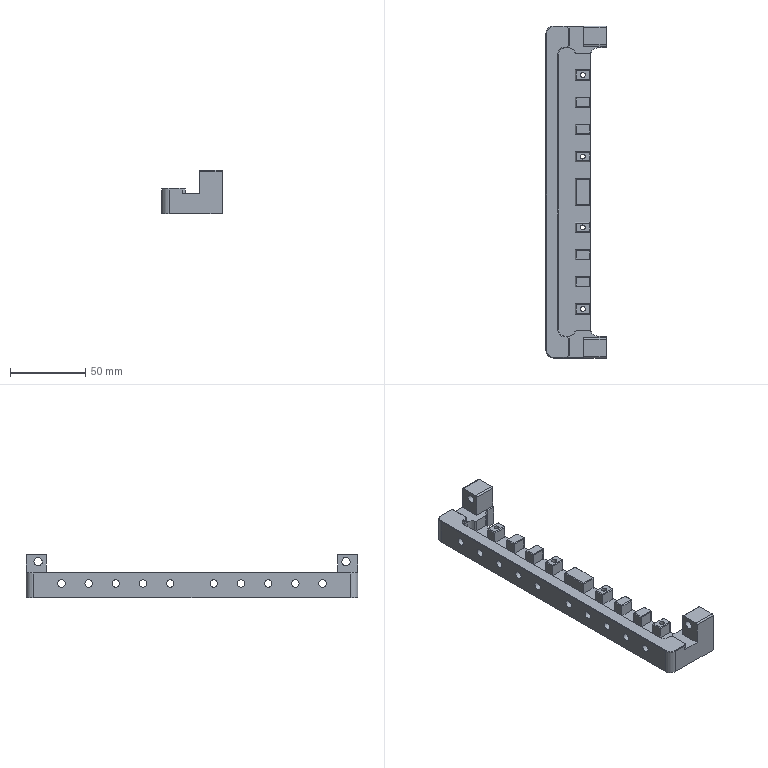Part | 1 solid | 187 faces | box 40 x 220 x 29 mm | volume 76343 mm3 | plane 107 | cylinder 54 | cone 26 | commonest cylinder face diameters 2 x26 5 x10 3.3 x4 4 x4 8 x4 10 x4